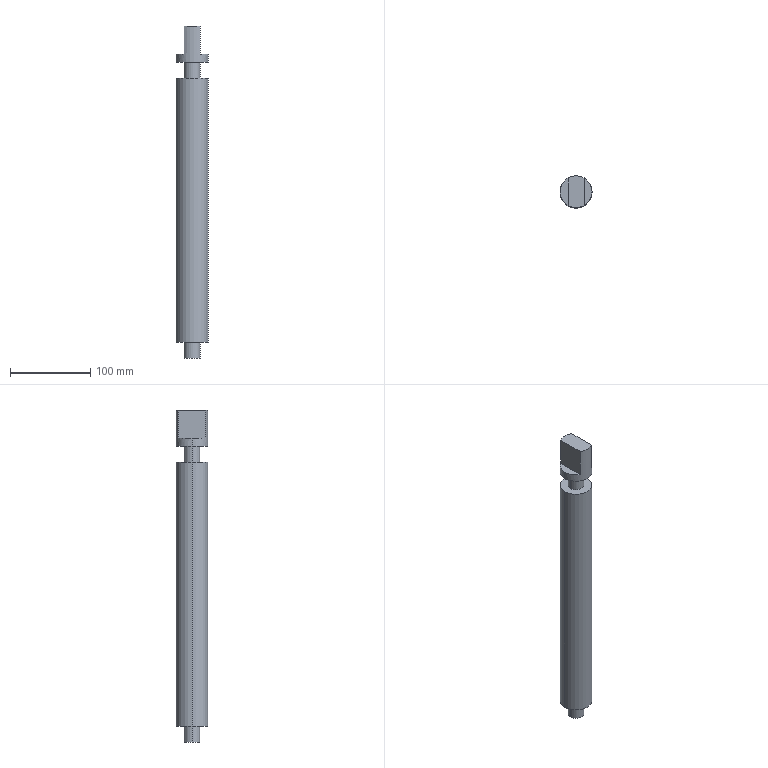Part | SolidWorks | 1 solid | 17 faces | box 40 x 40 x 415 mm | volume 466608 mm3 | plane 9 | cylinder 8 | commonest cylinder face diameters 20 x4 40 x4
STEP:
#1=CARTESIAN_POINT('',(-10.,0.,-185.));
#2=VERTEX_POINT('',#1);
#3=CARTESIAN_POINT('',(10.,0.,-185.));
#4=VERTEX_POINT('',#3);
#5=CARTESIAN_POINT('',(0.,0.,-185.));
#6=DIRECTION('',(0.,0.,-1.));
#7=DIRECTION('',(-1.,0.,0.));
#8=AXIS2_PLACEMENT_3D('',#5,#6,#7);
#9=CIRCLE('',#8,10.);
#10=EDGE_CURVE('',#2,#4,#9,.T.);
#11=ORIENTED_EDGE('',*,*,#10,.F.);
#12=CARTESIAN_POINT('',(-10.,0.,-165.));
#13=VERTEX_POINT('',#12);
#14=CARTESIAN_POINT('',(-10.,0.,-185.));
#15=DIRECTION('',(0.,0.,1.));
#16=VECTOR('',#15,1000.);
#17=LINE('',#14,#16);
#18=EDGE_CURVE('',#2,#13,#17,.T.);
#19=ORIENTED_EDGE('',*,*,#18,.T.);
#20=CARTESIAN_POINT('',(10.,0.,-165.));
#21=VERTEX_POINT('',#20);
#22=CARTESIAN_POINT('',(0.,0.,-165.));
#23=DIRECTION('',(0.,0.,-1.));
#24=DIRECTION('',(-1.,0.,0.));
#25=AXIS2_PLACEMENT_3D('',#22,#23,#24);
#26=CIRCLE('',#25,10.);
#27=EDGE_CURVE('',#13,#21,#26,.T.);
#28=ORIENTED_EDGE('',*,*,#27,.T.);
#29=CARTESIAN_POINT('',(10.,0.,-185.));
#30=DIRECTION('',(0.,0.,1.));
#31=VECTOR('',#30,1000.);
#32=LINE('',#29,#31);
#33=EDGE_CURVE('',#4,#21,#32,.T.);
#34=ORIENTED_EDGE('',*,*,#33,.F.);
#35=EDGE_LOOP('',(#11,#19,#28,#34));
#36=FACE_OUTER_BOUND('',#35,.T.);
#37=CARTESIAN_POINT('',(0.,0.,-185.));
#38=DIRECTION('',(0.,0.,1.));
#39=DIRECTION('',(1.,0.,0.));
#40=AXIS2_PLACEMENT_3D('',#37,#38,#39);
#41=CYLINDRICAL_SURFACE('',#40,10.);
#42=ADVANCED_FACE('',(#36),#41,.T.);
#43=CARTESIAN_POINT('',(20.,0.,165.));
#44=VERTEX_POINT('',#43);
#45=CARTESIAN_POINT('',(-20.,0.,165.));
#46=VERTEX_POINT('',#45);
#47=CARTESIAN_POINT('',(0.,0.,165.));
#48=DIRECTION('',(0.,0.,1.));
#49=DIRECTION('',(1.,0.,0.));
#50=AXIS2_PLACEMENT_3D('',#47,#48,#49);
#51=CIRCLE('',#50,20.);
#52=EDGE_CURVE('',#44,#46,#51,.T.);
#53=ORIENTED_EDGE('',*,*,#52,.F.);
#54=CARTESIAN_POINT('',(20.,0.,-165.));
#55=VERTEX_POINT('',#54);
#56=CARTESIAN_POINT('',(20.,0.,165.));
#57=DIRECTION('',(0.,0.,-1.));
#58=VECTOR('',#57,1000.);
#59=LINE('',#56,#58);
#60=EDGE_CURVE('',#44,#55,#59,.T.);
#61=ORIENTED_EDGE('',*,*,#60,.T.);
#62=CARTESIAN_POINT('',(-20.,0.,-165.));
#63=VERTEX_POINT('',#62);
#64=CARTESIAN_POINT('',(0.,0.,-165.));
#65=DIRECTION('',(0.,0.,1.));
#66=DIRECTION('',(1.,0.,0.));
#67=AXIS2_PLACEMENT_3D('',#64,#65,#66);
#68=CIRCLE('',#67,20.);
#69=EDGE_CURVE('',#55,#63,#68,.T.);
#70=ORIENTED_EDGE('',*,*,#69,.T.);
#71=CARTESIAN_POINT('',(-20.,0.,165.));
#72=DIRECTION('',(0.,0.,-1.));
#73=VECTOR('',#72,1000.);
#74=LINE('',#71,#73);
#75=EDGE_CURVE('',#46,#63,#74,.T.);
#76=ORIENTED_EDGE('',*,*,#75,.F.);
#77=EDGE_LOOP('',(#53,#61,#70,#76));
#78=FACE_OUTER_BOUND('',#77,.T.);
#79=CARTESIAN_POINT('',(0.,0.,165.));
#80=DIRECTION('',(0.,0.,-1.));
#81=DIRECTION('',(-1.,0.,0.));
#82=AXIS2_PLACEMENT_3D('',#79,#80,#81);
#83=CYLINDRICAL_SURFACE('',#82,20.);
#84=ADVANCED_FACE('',(#78),#83,.T.);
#85=CARTESIAN_POINT('',(10.,0.,185.));
#86=VERTEX_POINT('',#85);
#87=CARTESIAN_POINT('',(-10.,0.,185.));
#88=VERTEX_POINT('',#87);
#89=CARTESIAN_POINT('',(0.,0.,185.));
#90=DIRECTION('',(0.,0.,1.));
#91=DIRECTION('',(1.,0.,0.));
#92=AXIS2_PLACEMENT_3D('',#89,#90,#91);
#93=CIRCLE('',#92,10.);
#94=EDGE_CURVE('',#86,#88,#93,.T.);
#95=ORIENTED_EDGE('',*,*,#94,.F.);
#96=CARTESIAN_POINT('',(10.,0.,165.));
#97=VERTEX_POINT('',#96);
#98=CARTESIAN_POINT('',(10.,0.,230.));
#99=DIRECTION('',(0.,0.,-1.));
#100=VECTOR('',#99,1000.);
#101=LINE('',#98,#100);
#102=EDGE_CURVE('',#86,#97,#101,.T.);
#103=ORIENTED_EDGE('',*,*,#102,.T.);
#104=CARTESIAN_POINT('',(-10.,0.,165.));
#105=VERTEX_POINT('',#104);
#106=CARTESIAN_POINT('',(0.,0.,165.));
#107=DIRECTION('',(0.,0.,1.));
#108=DIRECTION('',(1.,0.,0.));
#109=AXIS2_PLACEMENT_3D('',#106,#107,#108);
#110=CIRCLE('',#109,10.);
#111=EDGE_CURVE('',#97,#105,#110,.T.);
#112=ORIENTED_EDGE('',*,*,#111,.T.);
#113=CARTESIAN_POINT('',(-10.,0.,230.));
#114=DIRECTION('',(0.,0.,-1.));
#115=VECTOR('',#114,1000.);
#116=LINE('',#113,#115);
#117=EDGE_CURVE('',#88,#105,#116,.T.);
#118=ORIENTED_EDGE('',*,*,#117,.F.);
#119=EDGE_LOOP('',(#95,#103,#112,#118));
#120=FACE_OUTER_BOUND('',#119,.T.);
#121=CARTESIAN_POINT('',(0.,0.,230.));
#122=DIRECTION('',(0.,0.,-1.));
#123=DIRECTION('',(-1.,0.,0.));
#124=AXIS2_PLACEMENT_3D('',#121,#122,#123);
#125=CYLINDRICAL_SURFACE('',#124,10.);
#126=ADVANCED_FACE('',(#120),#125,.T.);
#127=CARTESIAN_POINT('',(-20.,0.,185.));
#128=VERTEX_POINT('',#127);
#129=CARTESIAN_POINT('',(20.,0.,185.));
#130=VERTEX_POINT('',#129);
#131=CARTESIAN_POINT('',(0.,0.,185.));
#132=DIRECTION('',(0.,0.,-1.));
#133=DIRECTION('',(1.,0.,0.));
#134=AXIS2_PLACEMENT_3D('',#131,#132,#133);
#135=CIRCLE('',#134,20.);
#136=EDGE_CURVE('',#128,#130,#135,.T.);
#137=ORIENTED_EDGE('',*,*,#136,.F.);
#138=CARTESIAN_POINT('',(-20.,0.,195.));
#139=VERTEX_POINT('',#138);
#140=CARTESIAN_POINT('',(-20.,0.,128.431));
#141=DIRECTION('',(0.,0.,1.));
#142=VECTOR('',#141,1000.);
#143=LINE('',#140,#142);
#144=EDGE_CURVE('',#128,#139,#143,.T.);
#145=ORIENTED_EDGE('',*,*,#144,.T.);
#146=CARTESIAN_POINT('',(-10.,17.321,195.));
#147=VERTEX_POINT('',#146);
#148=CARTESIAN_POINT('',(0.,0.,195.));
#149=DIRECTION('',(0.,0.,-1.));
#150=DIRECTION('',(-1.,0.,0.));
#151=AXIS2_PLACEMENT_3D('',#148,#149,#150);
#152=CIRCLE('',#151,20.);
#153=EDGE_CURVE('',#139,#147,#152,.T.);
#154=ORIENTED_EDGE('',*,*,#153,.T.);
#155=CARTESIAN_POINT('',(-10.,17.321,230.));
#156=VERTEX_POINT('',#155);
#157=CARTESIAN_POINT('',(-10.,17.321,176.));
#158=DIRECTION('',(0.,0.,1.));
#159=VECTOR('',#158,1000.);
#160=LINE('',#157,#159);
#161=EDGE_CURVE('',#147,#156,#160,.T.);
#162=ORIENTED_EDGE('',*,*,#161,.T.);
#163=CARTESIAN_POINT('',(10.,17.321,230.));
#164=VERTEX_POINT('',#163);
#165=CARTESIAN_POINT('',(0.,0.,230.));
#166=DIRECTION('',(0.,0.,1.));
#167=DIRECTION('',(1.,0.,0.));
#168=AXIS2_PLACEMENT_3D('',#165,#166,#167);
#169=CIRCLE('',#168,20.);
#170=EDGE_CURVE('',#164,#156,#169,.T.);
#171=ORIENTED_EDGE('',*,*,#170,.F.);
#172=CARTESIAN_POINT('',(10.,17.321,195.));
#173=VERTEX_POINT('',#172);
#174=CARTESIAN_POINT('',(10.,17.321,176.));
#175=DIRECTION('',(0.,0.,1.));
#176=VECTOR('',#175,1000.);
#177=LINE('',#174,#176);
#178=EDGE_CURVE('',#173,#164,#177,.T.);
#179=ORIENTED_EDGE('',*,*,#178,.F.);
#180=CARTESIAN_POINT('',(20.,0.,195.));
#181=VERTEX_POINT('',#180);
#182=CARTESIAN_POINT('',(0.,0.,195.));
#183=DIRECTION('',(0.,0.,-1.));
#184=DIRECTION('',(-1.,0.,0.));
#185=AXIS2_PLACEMENT_3D('',#182,#183,#184);
#186=CIRCLE('',#185,20.);
#187=EDGE_CURVE('',#173,#181,#186,.T.);
#188=ORIENTED_EDGE('',*,*,#187,.T.);
#189=CARTESIAN_POINT('',(20.,0.,128.431));
#190=DIRECTION('',(0.,0.,1.));
#191=VECTOR('',#190,1000.);
#192=LINE('',#189,#191);
#193=EDGE_CURVE('',#130,#181,#192,.T.);
#194=ORIENTED_EDGE('',*,*,#193,.F.);
#195=EDGE_LOOP('',(#137,#145,#154,#162,#171,#179,#188,#194));
#196=FACE_OUTER_BOUND('',#195,.T.);
#197=CARTESIAN_POINT('',(0.,0.,128.431));
#198=DIRECTION('',(0.,0.,1.));
#199=DIRECTION('',(1.,0.,0.));
#200=AXIS2_PLACEMENT_3D('',#197,#198,#199);
#201=CYLINDRICAL_SURFACE('',#200,20.);
#202=ADVANCED_FACE('',(#196),#201,.T.);
#203=ORIENTED_EDGE('',*,*,#161,.F.);
#204=CARTESIAN_POINT('',(-10.,-17.321,195.));
#205=VERTEX_POINT('',#204);
#206=CARTESIAN_POINT('',(-10.,0.,195.));
#207=DIRECTION('',(0.,-1.,0.));
#208=VECTOR('',#207,1000.);
#209=LINE('',#206,#208);
#210=EDGE_CURVE('',#147,#205,#209,.T.);
#211=ORIENTED_EDGE('',*,*,#210,.T.);
#212=CARTESIAN_POINT('',(-10.,-17.321,230.));
#213=VERTEX_POINT('',#212);
#214=CARTESIAN_POINT('',(-10.,-17.321,176.));
#215=DIRECTION('',(0.,0.,1.));
#216=VECTOR('',#215,1000.);
#217=LINE('',#214,#216);
#218=EDGE_CURVE('',#205,#213,#217,.T.);
#219=ORIENTED_EDGE('',*,*,#218,.T.);
#220=CARTESIAN_POINT('',(-10.,0.,230.));
#221=DIRECTION('',(0.,-1.,0.));
#222=VECTOR('',#221,1000.);
#223=LINE('',#220,#222);
#224=EDGE_CURVE('',#156,#213,#223,.T.);
#225=ORIENTED_EDGE('',*,*,#224,.F.);
#226=EDGE_LOOP('',(#203,#211,#219,#225));
#227=FACE_OUTER_BOUND('',#226,.T.);
#228=CARTESIAN_POINT('',(-10.,0.,176.));
#229=DIRECTION('',(-1.,0.,0.));
#230=DIRECTION('',(0.,0.,1.));
#231=AXIS2_PLACEMENT_3D('',#228,#229,#230);
#232=PLANE('',#231);
#233=ADVANCED_FACE('',(#227),#232,.T.);
#234=CARTESIAN_POINT('',(10.,-17.321,195.));
#235=VERTEX_POINT('',#234);
#236=CARTESIAN_POINT('',(10.,0.,195.));
#237=DIRECTION('',(0.,-1.,0.));
#238=VECTOR('',#237,1000.);
#239=LINE('',#236,#238);
#240=EDGE_CURVE('',#173,#235,#239,.T.);
#241=ORIENTED_EDGE('',*,*,#240,.F.);
#242=ORIENTED_EDGE('',*,*,#178,.T.);
#243=CARTESIAN_POINT('',(10.,-17.321,230.));
#244=VERTEX_POINT('',#243);
#245=CARTESIAN_POINT('',(10.,0.,230.));
#246=DIRECTION('',(0.,-1.,0.));
#247=VECTOR('',#246,1000.);
#248=LINE('',#245,#247);
#249=EDGE_CURVE('',#164,#244,#248,.T.);
#250=ORIENTED_EDGE('',*,*,#249,.T.);
#251=CARTESIAN_POINT('',(10.,-17.321,176.));
#252=DIRECTION('',(0.,0.,1.));
#253=VECTOR('',#252,1000.);
#254=LINE('',#251,#253);
#255=EDGE_CURVE('',#235,#244,#254,.T.);
#256=ORIENTED_EDGE('',*,*,#255,.F.);
#257=EDGE_LOOP('',(#241,#242,#250,#256));
#258=FACE_OUTER_BOUND('',#257,.T.);
#259=CARTESIAN_POINT('',(10.,0.,176.));
#260=DIRECTION('',(-1.,0.,0.));
#261=DIRECTION('',(0.,0.,1.));
#262=AXIS2_PLACEMENT_3D('',#259,#260,#261);
#263=PLANE('',#262);
#264=ADVANCED_FACE('',(#258),#263,.F.);
#265=ORIENTED_EDGE('',*,*,#144,.F.);
#266=CARTESIAN_POINT('',(0.,0.,185.));
#267=DIRECTION('',(0.,0.,-1.));
#268=DIRECTION('',(1.,0.,0.));
#269=AXIS2_PLACEMENT_3D('',#266,#267,#268);
#270=CIRCLE('',#269,20.);
#271=EDGE_CURVE('',#130,#128,#270,.T.);
#272=ORIENTED_EDGE('',*,*,#271,.F.);
#273=ORIENTED_EDGE('',*,*,#193,.T.);
#274=CARTESIAN_POINT('',(0.,0.,195.));
#275=DIRECTION('',(0.,0.,-1.));
#276=DIRECTION('',(-1.,0.,0.));
#277=AXIS2_PLACEMENT_3D('',#274,#275,#276);
#278=CIRCLE('',#277,20.);
#279=EDGE_CURVE('',#181,#235,#278,.T.);
#280=ORIENTED_EDGE('',*,*,#279,.T.);
#281=ORIENTED_EDGE('',*,*,#255,.T.);
#282=CARTESIAN_POINT('',(0.,0.,230.));
#283=DIRECTION('',(0.,0.,1.));
#284=DIRECTION('',(1.,0.,0.));
#285=AXIS2_PLACEMENT_3D('',#282,#283,#284);
#286=CIRCLE('',#285,20.);
#287=EDGE_CURVE('',#213,#244,#286,.T.);
#288=ORIENTED_EDGE('',*,*,#287,.F.);
#289=ORIENTED_EDGE('',*,*,#218,.F.);
#290=CARTESIAN_POINT('',(0.,0.,195.));
#291=DIRECTION('',(0.,0.,-1.));
#292=DIRECTION('',(-1.,0.,0.));
#293=AXIS2_PLACEMENT_3D('',#290,#291,#292);
#294=CIRCLE('',#293,20.);
#295=EDGE_CURVE('',#205,#139,#294,.T.);
#296=ORIENTED_EDGE('',*,*,#295,.T.);
#297=EDGE_LOOP('',(#265,#272,#273,#280,#281,#288,#289,#296));
#298=FACE_OUTER_BOUND('',#297,.T.);
#299=CARTESIAN_POINT('',(0.,0.,128.431));
#300=DIRECTION('',(0.,0.,1.));
#301=DIRECTION('',(1.,0.,0.));
#302=AXIS2_PLACEMENT_3D('',#299,#300,#301);
#303=CYLINDRICAL_SURFACE('',#302,20.);
#304=ADVANCED_FACE('',(#298),#303,.T.);
#305=CARTESIAN_POINT('',(0.,0.,185.));
#306=DIRECTION('',(0.,0.,1.));
#307=DIRECTION('',(1.,0.,0.));
#308=AXIS2_PLACEMENT_3D('',#305,#306,#307);
#309=CIRCLE('',#308,10.);
#310=EDGE_CURVE('',#88,#86,#309,.T.);
#311=ORIENTED_EDGE('',*,*,#310,.T.);
#312=ORIENTED_EDGE('',*,*,#94,.T.);
#313=EDGE_LOOP('',(#311,#312));
#314=FACE_BOUND('',#313,.T.);
#315=ORIENTED_EDGE('',*,*,#271,.T.);
#316=ORIENTED_EDGE('',*,*,#136,.T.);
#317=EDGE_LOOP('',(#315,#316));
#318=FACE_OUTER_BOUND('',#317,.T.);
#319=CARTESIAN_POINT('',(0.,0.,185.));
#320=DIRECTION('',(0.,0.,1.));
#321=DIRECTION('',(1.,0.,0.));
#322=AXIS2_PLACEMENT_3D('',#319,#320,#321);
#323=PLANE('',#322);
#324=ADVANCED_FACE('',(#314,#318),#323,.F.);
#325=ORIENTED_EDGE('',*,*,#249,.F.);
#326=ORIENTED_EDGE('',*,*,#170,.T.);
#327=ORIENTED_EDGE('',*,*,#224,.T.);
#328=ORIENTED_EDGE('',*,*,#287,.T.);
#329=EDGE_LOOP('',(#325,#326,#327,#328));
#330=FACE_OUTER_BOUND('',#329,.T.);
#331=CARTESIAN_POINT('',(0.,0.,230.));
#332=DIRECTION('',(0.,0.,1.));
#333=DIRECTION('',(1.,0.,0.));
#334=AXIS2_PLACEMENT_3D('',#331,#332,#333);
#335=PLANE('',#334);
#336=ADVANCED_FACE('',(#330),#335,.T.);
#337=ORIENTED_EDGE('',*,*,#102,.F.);
#338=ORIENTED_EDGE('',*,*,#310,.F.);
#339=ORIENTED_EDGE('',*,*,#117,.T.);
#340=CARTESIAN_POINT('',(0.,0.,165.));
#341=DIRECTION('',(0.,0.,1.));
#342=DIRECTION('',(1.,0.,0.));
#343=AXIS2_PLACEMENT_3D('',#340,#341,#342);
#344=CIRCLE('',#343,10.);
#345=EDGE_CURVE('',#105,#97,#344,.T.);
#346=ORIENTED_EDGE('',*,*,#345,.T.);
#347=EDGE_LOOP('',(#337,#338,#339,#346));
#348=FACE_OUTER_BOUND('',#347,.T.);
#349=CARTESIAN_POINT('',(0.,0.,230.));
#350=DIRECTION('',(0.,0.,-1.));
#351=DIRECTION('',(-1.,0.,0.));
#352=AXIS2_PLACEMENT_3D('',#349,#350,#351);
#353=CYLINDRICAL_SURFACE('',#352,10.);
#354=ADVANCED_FACE('',(#348),#353,.T.);
#355=ORIENTED_EDGE('',*,*,#60,.F.);
#356=CARTESIAN_POINT('',(0.,0.,165.));
#357=DIRECTION('',(0.,0.,1.));
#358=DIRECTION('',(1.,0.,0.));
#359=AXIS2_PLACEMENT_3D('',#356,#357,#358);
#360=CIRCLE('',#359,20.);
#361=EDGE_CURVE('',#46,#44,#360,.T.);
#362=ORIENTED_EDGE('',*,*,#361,.F.);
#363=ORIENTED_EDGE('',*,*,#75,.T.);
#364=CARTESIAN_POINT('',(0.,0.,-165.));
#365=DIRECTION('',(0.,0.,1.));
#366=DIRECTION('',(1.,0.,0.));
#367=AXIS2_PLACEMENT_3D('',#364,#365,#366);
#368=CIRCLE('',#367,20.);
#369=EDGE_CURVE('',#63,#55,#368,.T.);
#370=ORIENTED_EDGE('',*,*,#369,.T.);
#371=EDGE_LOOP('',(#355,#362,#363,#370));
#372=FACE_OUTER_BOUND('',#371,.T.);
#373=CARTESIAN_POINT('',(0.,0.,165.));
#374=DIRECTION('',(0.,0.,-1.));
#375=DIRECTION('',(-1.,0.,0.));
#376=AXIS2_PLACEMENT_3D('',#373,#374,#375);
#377=CYLINDRICAL_SURFACE('',#376,20.);
#378=ADVANCED_FACE('',(#372),#377,.T.);
#379=ORIENTED_EDGE('',*,*,#345,.F.);
#380=ORIENTED_EDGE('',*,*,#111,.F.);
#381=EDGE_LOOP('',(#379,#380));
#382=FACE_BOUND('',#381,.T.);
#383=ORIENTED_EDGE('',*,*,#361,.T.);
#384=ORIENTED_EDGE('',*,*,#52,.T.);
#385=EDGE_LOOP('',(#383,#384));
#386=FACE_OUTER_BOUND('',#385,.T.);
#387=CARTESIAN_POINT('',(0.,0.,165.));
#388=DIRECTION('',(0.,0.,1.));
#389=DIRECTION('',(1.,0.,0.));
#390=AXIS2_PLACEMENT_3D('',#387,#388,#389);
#391=PLANE('',#390);
#392=ADVANCED_FACE('',(#382,#386),#391,.T.);
#393=CARTESIAN_POINT('',(0.,0.,-165.));
#394=DIRECTION('',(0.,0.,-1.));
#395=DIRECTION('',(-1.,0.,0.));
#396=AXIS2_PLACEMENT_3D('',#393,#394,#395);
#397=CIRCLE('',#396,10.);
#398=EDGE_CURVE('',#21,#13,#397,.T.);
#399=ORIENTED_EDGE('',*,*,#398,.F.);
#400=ORIENTED_EDGE('',*,*,#27,.F.);
#401=EDGE_LOOP('',(#399,#400));
#402=FACE_BOUND('',#401,.T.);
#403=ORIENTED_EDGE('',*,*,#369,.F.);
#404=ORIENTED_EDGE('',*,*,#69,.F.);
#405=EDGE_LOOP('',(#403,#404));
#406=FACE_OUTER_BOUND('',#405,.T.);
#407=CARTESIAN_POINT('',(0.,0.,-165.));
#408=DIRECTION('',(0.,0.,1.));
#409=DIRECTION('',(1.,0.,0.));
#410=AXIS2_PLACEMENT_3D('',#407,#408,#409);
#411=PLANE('',#410);
#412=ADVANCED_FACE('',(#402,#406),#411,.F.);
#413=ORIENTED_EDGE('',*,*,#18,.F.);
#414=CARTESIAN_POINT('',(0.,0.,-185.));
#415=DIRECTION('',(0.,0.,-1.));
#416=DIRECTION('',(-1.,0.,0.));
#417=AXIS2_PLACEMENT_3D('',#414,#415,#416);
#418=CIRCLE('',#417,10.);
#419=EDGE_CURVE('',#4,#2,#418,.T.);
#420=ORIENTED_EDGE('',*,*,#419,.F.);
#421=ORIENTED_EDGE('',*,*,#33,.T.);
#422=ORIENTED_EDGE('',*,*,#398,.T.);
#423=EDGE_LOOP('',(#413,#420,#421,#422));
#424=FACE_OUTER_BOUND('',#423,.T.);
#425=CARTESIAN_POINT('',(0.,0.,-185.));
#426=DIRECTION('',(0.,0.,1.));
#427=DIRECTION('',(1.,0.,0.));
#428=AXIS2_PLACEMENT_3D('',#425,#426,#427);
#429=CYLINDRICAL_SURFACE('',#428,10.);
#430=ADVANCED_FACE('',(#424),#429,.T.);
#431=ORIENTED_EDGE('',*,*,#419,.T.);
#432=ORIENTED_EDGE('',*,*,#10,.T.);
#433=EDGE_LOOP('',(#431,#432));
#434=FACE_OUTER_BOUND('',#433,.T.);
#435=CARTESIAN_POINT('',(0.,0.,-185.));
#436=DIRECTION('',(0.,0.,-1.));
#437=DIRECTION('',(-1.,0.,0.));
#438=AXIS2_PLACEMENT_3D('',#435,#436,#437);
#439=PLANE('',#438);
#440=ADVANCED_FACE('',(#434),#439,.T.);
#441=ORIENTED_EDGE('',*,*,#187,.F.);
#442=ORIENTED_EDGE('',*,*,#240,.T.);
#443=ORIENTED_EDGE('',*,*,#279,.F.);
#444=EDGE_LOOP('',(#441,#442,#443));
#445=FACE_OUTER_BOUND('',#444,.T.);
#446=CARTESIAN_POINT('',(0.,0.,195.));
#447=DIRECTION('',(0.,0.,-1.));
#448=DIRECTION('',(-1.,0.,0.));
#449=AXIS2_PLACEMENT_3D('',#446,#447,#448);
#450=PLANE('',#449);
#451=ADVANCED_FACE('',(#445),#450,.F.);
#452=ORIENTED_EDGE('',*,*,#210,.F.);
#453=ORIENTED_EDGE('',*,*,#153,.F.);
#454=ORIENTED_EDGE('',*,*,#295,.F.);
#455=EDGE_LOOP('',(#452,#453,#454));
#456=FACE_OUTER_BOUND('',#455,.T.);
#457=CARTESIAN_POINT('',(0.,0.,195.));
#458=DIRECTION('',(0.,0.,-1.));
#459=DIRECTION('',(-1.,0.,0.));
#460=AXIS2_PLACEMENT_3D('',#457,#458,#459);
#461=PLANE('',#460);
#462=ADVANCED_FACE('',(#456),#461,.F.);
#463=CLOSED_SHELL('',(#42,#84,#126,#202,#233,#264,#304,#324,#336,#354,#378,#392,#412,#430,#440,#451,#462));
#464=MANIFOLD_SOLID_BREP('',#463);
#465=CARTESIAN_POINT('',(0.,0.,0.));
#466=DIRECTION('',(0.,0.,1.));
#467=DIRECTION('',(1.,0.,0.));
#468=AXIS2_PLACEMENT_3D('',#465,#466,#467);
#469=(LENGTH_UNIT()NAMED_UNIT(*)SI_UNIT(.MILLI.,.METRE.));
#470=UNCERTAINTY_MEASURE_WITH_UNIT(LENGTH_MEASURE(0.00001),#469,'','');
#471=(NAMED_UNIT(*)PLANE_ANGLE_UNIT()SI_UNIT($,.RADIAN.));
#472=(NAMED_UNIT(*)SI_UNIT($,.STERADIAN.)SOLID_ANGLE_UNIT());
#473=(GEOMETRIC_REPRESENTATION_CONTEXT(3)GLOBAL_UNCERTAINTY_ASSIGNED_CONTEXT((#470))GLOBAL_UNIT_ASSIGNED_CONTEXT((#469,#471,#472))REPRESENTATION_CONTEXT('',''));
#474=ADVANCED_BREP_SHAPE_REPRESENTATION('',(#464,#468),#473);